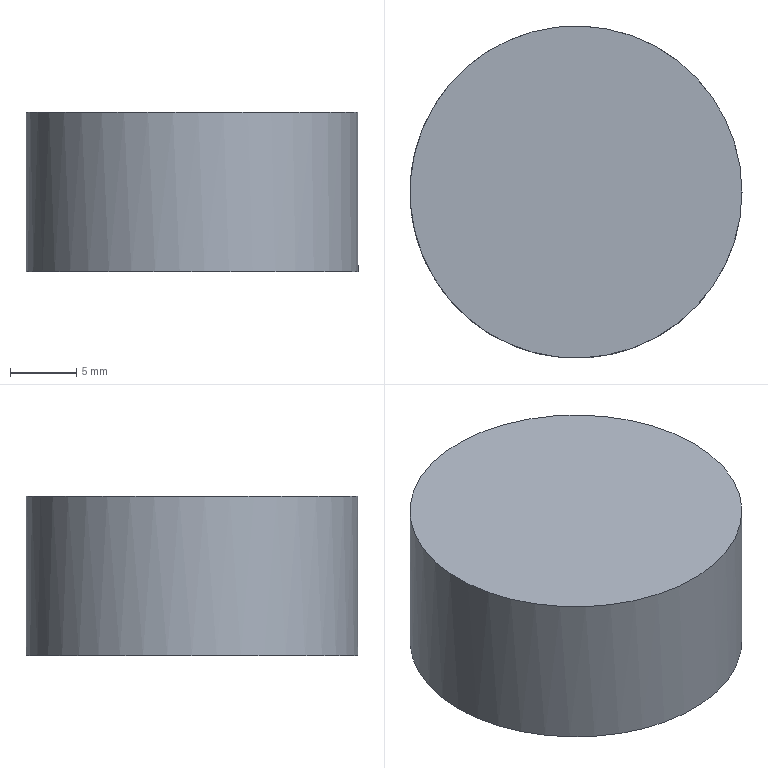Part | STEP file | solid 112 | 1 solid | 3 faces | box 25 x 25 x 12 mm | volume 5890 mm3 | plane 2 | cylinder 1 | commonest cylinder face diameters 25 x1